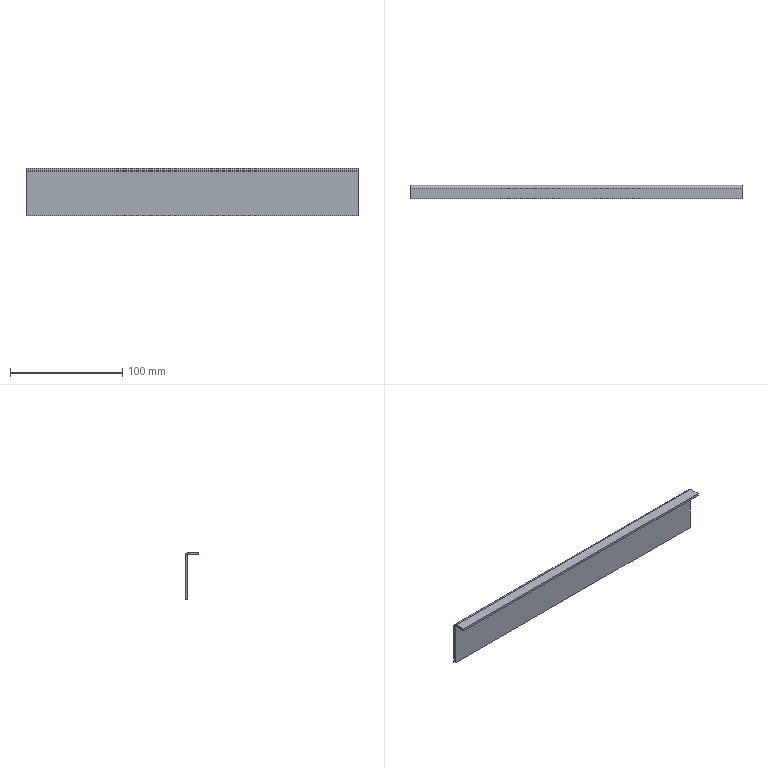Part | NX | 1 solid | 14 faces | box 296 x 12 x 42 mm | volume 30343 mm3 | plane 12 | cylinder 2 | commonest cylinder face diameters 1.473 x1 5.473 x1
STEP:
#1=CARTESIAN_POINT('',(-148.,-2.,-20.));
#2=VERTEX_POINT('',#1);
#3=CARTESIAN_POINT('',(-148.,-2.,19.263));
#4=VERTEX_POINT('',#3);
#5=CARTESIAN_POINT('',(-148.,-2.,20.));
#6=DIRECTION('',(0.,0.,1.));
#7=VECTOR('',#6,1000.);
#8=LINE('',#5,#7);
#9=EDGE_CURVE('',#2,#4,#8,.T.);
#10=ORIENTED_EDGE('',*,*,#9,.T.);
#11=CARTESIAN_POINT('',(-148.,0.,19.263));
#12=VERTEX_POINT('',#11);
#13=CARTESIAN_POINT('',(-148.,-2.,19.263));
#14=DIRECTION('',(0.,1.,0.));
#15=VECTOR('',#14,1000.);
#16=LINE('',#13,#15);
#17=EDGE_CURVE('',#4,#12,#16,.T.);
#18=ORIENTED_EDGE('',*,*,#17,.T.);
#19=CARTESIAN_POINT('',(-148.,0.,-20.));
#20=VERTEX_POINT('',#19);
#21=CARTESIAN_POINT('',(-148.,0.,20.));
#22=DIRECTION('',(0.,0.,1.));
#23=VECTOR('',#22,1000.);
#24=LINE('',#21,#23);
#25=EDGE_CURVE('',#20,#12,#24,.T.);
#26=ORIENTED_EDGE('',*,*,#25,.F.);
#27=CARTESIAN_POINT('',(-148.,-2.,-20.));
#28=DIRECTION('',(0.,1.,0.));
#29=VECTOR('',#28,1000.);
#30=LINE('',#27,#29);
#31=EDGE_CURVE('',#2,#20,#30,.T.);
#32=ORIENTED_EDGE('',*,*,#31,.F.);
#33=EDGE_LOOP('',(#10,#18,#26,#32));
#34=FACE_BOUND('',#33,.T.);
#35=CARTESIAN_POINT('',(-148.,-2.,20.));
#36=DIRECTION('',(-1.,0.,0.));
#37=DIRECTION('',(0.,0.,1.));
#38=AXIS2_PLACEMENT_3D('',#35,#36,#37);
#39=PLANE('',#38);
#40=ADVANCED_FACE('',(#34),#39,.T.);
#41=CARTESIAN_POINT('',(148.,-2.,19.263));
#42=VERTEX_POINT('',#41);
#43=CARTESIAN_POINT('',(148.,-2.,-20.));
#44=VERTEX_POINT('',#43);
#45=CARTESIAN_POINT('',(148.,-2.,20.));
#46=DIRECTION('',(0.,0.,-1.));
#47=VECTOR('',#46,1000.);
#48=LINE('',#45,#47);
#49=EDGE_CURVE('',#42,#44,#48,.T.);
#50=ORIENTED_EDGE('',*,*,#49,.F.);
#51=CARTESIAN_POINT('',(-148.,-2.,19.263));
#52=DIRECTION('',(-1.,0.,0.));
#53=VECTOR('',#52,1000.);
#54=LINE('',#51,#53);
#55=EDGE_CURVE('',#4,#42,#54,.F.);
#56=ORIENTED_EDGE('',*,*,#55,.F.);
#57=ORIENTED_EDGE('',*,*,#9,.F.);
#58=CARTESIAN_POINT('',(-148.,-2.,-20.));
#59=DIRECTION('',(-1.,0.,0.));
#60=VECTOR('',#59,1000.);
#61=LINE('',#58,#60);
#62=EDGE_CURVE('',#44,#2,#61,.T.);
#63=ORIENTED_EDGE('',*,*,#62,.F.);
#64=EDGE_LOOP('',(#50,#56,#57,#63));
#65=FACE_BOUND('',#64,.T.);
#66=CARTESIAN_POINT('',(0.,-2.,0.));
#67=DIRECTION('',(0.,-1.,0.));
#68=DIRECTION('',(0.,0.,-1.));
#69=AXIS2_PLACEMENT_3D('',#66,#67,#68);
#70=PLANE('',#69);
#71=ADVANCED_FACE('',(#65),#70,.T.);
#72=CARTESIAN_POINT('',(148.,0.,19.263));
#73=VERTEX_POINT('',#72);
#74=CARTESIAN_POINT('',(-148.,0.,19.263));
#75=DIRECTION('',(-1.,0.,0.));
#76=VECTOR('',#75,1000.);
#77=LINE('',#74,#76);
#78=EDGE_CURVE('',#12,#73,#77,.F.);
#79=ORIENTED_EDGE('',*,*,#78,.T.);
#80=CARTESIAN_POINT('',(148.,0.,-20.));
#81=VERTEX_POINT('',#80);
#82=CARTESIAN_POINT('',(148.,0.,20.));
#83=DIRECTION('',(0.,0.,-1.));
#84=VECTOR('',#83,1000.);
#85=LINE('',#82,#84);
#86=EDGE_CURVE('',#73,#81,#85,.T.);
#87=ORIENTED_EDGE('',*,*,#86,.T.);
#88=CARTESIAN_POINT('',(-148.,0.,-20.));
#89=DIRECTION('',(-1.,0.,0.));
#90=VECTOR('',#89,1000.);
#91=LINE('',#88,#90);
#92=EDGE_CURVE('',#81,#20,#91,.T.);
#93=ORIENTED_EDGE('',*,*,#92,.T.);
#94=ORIENTED_EDGE('',*,*,#25,.T.);
#95=EDGE_LOOP('',(#79,#87,#93,#94));
#96=FACE_BOUND('',#95,.T.);
#97=CARTESIAN_POINT('',(0.,0.,0.));
#98=DIRECTION('',(0.,-1.,0.));
#99=DIRECTION('',(0.,0.,-1.));
#100=AXIS2_PLACEMENT_3D('',#97,#98,#99);
#101=PLANE('',#100);
#102=ADVANCED_FACE('',(#96),#101,.F.);
#103=CARTESIAN_POINT('',(148.,-2.,19.263));
#104=DIRECTION('',(0.,1.,0.));
#105=VECTOR('',#104,1000.);
#106=LINE('',#103,#105);
#107=EDGE_CURVE('',#42,#73,#106,.T.);
#108=ORIENTED_EDGE('',*,*,#107,.F.);
#109=ORIENTED_EDGE('',*,*,#49,.T.);
#110=CARTESIAN_POINT('',(148.,-2.,-20.));
#111=DIRECTION('',(0.,1.,0.));
#112=VECTOR('',#111,1000.);
#113=LINE('',#110,#112);
#114=EDGE_CURVE('',#44,#81,#113,.T.);
#115=ORIENTED_EDGE('',*,*,#114,.T.);
#116=ORIENTED_EDGE('',*,*,#86,.F.);
#117=EDGE_LOOP('',(#108,#109,#115,#116));
#118=FACE_BOUND('',#117,.T.);
#119=CARTESIAN_POINT('',(148.,-2.,20.));
#120=DIRECTION('',(1.,0.,0.));
#121=DIRECTION('',(0.,0.,-1.));
#122=AXIS2_PLACEMENT_3D('',#119,#120,#121);
#123=PLANE('',#122);
#124=ADVANCED_FACE('',(#118),#123,.T.);
#125=ORIENTED_EDGE('',*,*,#92,.F.);
#126=ORIENTED_EDGE('',*,*,#114,.F.);
#127=ORIENTED_EDGE('',*,*,#62,.T.);
#128=ORIENTED_EDGE('',*,*,#31,.T.);
#129=EDGE_LOOP('',(#125,#126,#127,#128));
#130=FACE_BOUND('',#129,.T.);
#131=CARTESIAN_POINT('',(-148.,-2.,-20.));
#132=DIRECTION('',(0.,0.,-1.));
#133=DIRECTION('',(-1.,0.,0.));
#134=AXIS2_PLACEMENT_3D('',#131,#132,#133);
#135=PLANE('',#134);
#136=ADVANCED_FACE('',(#130),#135,.T.);
#137=CARTESIAN_POINT('',(148.,-2.737,20.));
#138=VERTEX_POINT('',#137);
#139=CARTESIAN_POINT('',(148.,-2.737,22.));
#140=VERTEX_POINT('',#139);
#141=CARTESIAN_POINT('',(148.,-2.737,20.));
#142=DIRECTION('',(0.,0.,1.));
#143=VECTOR('',#142,1000.);
#144=LINE('',#141,#143);
#145=EDGE_CURVE('',#138,#140,#144,.T.);
#146=ORIENTED_EDGE('',*,*,#145,.F.);
#147=CARTESIAN_POINT('',(148.,-2.737,19.263));
#148=DIRECTION('',(-1.,0.,0.));
#149=DIRECTION('',(0.,0.,1.));
#150=AXIS2_PLACEMENT_3D('',#147,#148,#149);
#151=CIRCLE('',#150,0.7366);
#152=EDGE_CURVE('',#42,#138,#151,.F.);
#153=ORIENTED_EDGE('',*,*,#152,.F.);
#154=ORIENTED_EDGE('',*,*,#107,.T.);
#155=CARTESIAN_POINT('',(148.,-2.737,19.263));
#156=DIRECTION('',(-1.,0.,0.));
#157=DIRECTION('',(0.,0.,1.));
#158=AXIS2_PLACEMENT_3D('',#155,#156,#157);
#159=CIRCLE('',#158,2.737);
#160=EDGE_CURVE('',#73,#140,#159,.F.);
#161=ORIENTED_EDGE('',*,*,#160,.T.);
#162=EDGE_LOOP('',(#146,#153,#154,#161));
#163=FACE_BOUND('',#162,.T.);
#164=CARTESIAN_POINT('',(148.,-2.737,19.263));
#165=DIRECTION('',(1.,0.,0.));
#166=DIRECTION('',(0.,0.,-1.));
#167=AXIS2_PLACEMENT_3D('',#164,#165,#166);
#168=PLANE('',#167);
#169=ADVANCED_FACE('',(#163),#168,.T.);
#170=CARTESIAN_POINT('',(-148.,-2.737,20.));
#171=VERTEX_POINT('',#170);
#172=CARTESIAN_POINT('',(-148.,-2.737,19.263));
#173=DIRECTION('',(-1.,0.,0.));
#174=DIRECTION('',(0.,0.,1.));
#175=AXIS2_PLACEMENT_3D('',#172,#173,#174);
#176=CIRCLE('',#175,0.7366);
#177=EDGE_CURVE('',#171,#4,#176,.T.);
#178=ORIENTED_EDGE('',*,*,#177,.F.);
#179=CARTESIAN_POINT('',(-148.,-2.737,22.));
#180=VERTEX_POINT('',#179);
#181=CARTESIAN_POINT('',(-148.,-2.737,20.));
#182=DIRECTION('',(0.,0.,1.));
#183=VECTOR('',#182,1000.);
#184=LINE('',#181,#183);
#185=EDGE_CURVE('',#171,#180,#184,.T.);
#186=ORIENTED_EDGE('',*,*,#185,.T.);
#187=CARTESIAN_POINT('',(-148.,-2.737,19.263));
#188=DIRECTION('',(-1.,0.,0.));
#189=DIRECTION('',(0.,0.,1.));
#190=AXIS2_PLACEMENT_3D('',#187,#188,#189);
#191=CIRCLE('',#190,2.737);
#192=EDGE_CURVE('',#180,#12,#191,.T.);
#193=ORIENTED_EDGE('',*,*,#192,.T.);
#194=ORIENTED_EDGE('',*,*,#17,.F.);
#195=EDGE_LOOP('',(#178,#186,#193,#194));
#196=FACE_BOUND('',#195,.T.);
#197=CARTESIAN_POINT('',(-148.,-2.737,19.263));
#198=DIRECTION('',(1.,0.,0.));
#199=DIRECTION('',(0.,0.,-1.));
#200=AXIS2_PLACEMENT_3D('',#197,#198,#199);
#201=PLANE('',#200);
#202=ADVANCED_FACE('',(#196),#201,.F.);
#203=ORIENTED_EDGE('',*,*,#78,.F.);
#204=ORIENTED_EDGE('',*,*,#192,.F.);
#205=CARTESIAN_POINT('',(0.,-2.737,22.));
#206=DIRECTION('',(-1.,0.,0.));
#207=VECTOR('',#206,1000.);
#208=LINE('',#205,#207);
#209=EDGE_CURVE('',#140,#180,#208,.T.);
#210=ORIENTED_EDGE('',*,*,#209,.F.);
#211=ORIENTED_EDGE('',*,*,#160,.F.);
#212=EDGE_LOOP('',(#203,#204,#210,#211));
#213=FACE_BOUND('',#212,.T.);
#214=CARTESIAN_POINT('',(-148.,-2.737,19.263));
#215=DIRECTION('',(-1.,0.,0.));
#216=DIRECTION('',(0.,0.,1.));
#217=AXIS2_PLACEMENT_3D('',#214,#215,#216);
#218=CYLINDRICAL_SURFACE('',#217,2.737);
#219=ADVANCED_FACE('',(#213),#218,.T.);
#220=ORIENTED_EDGE('',*,*,#55,.T.);
#221=ORIENTED_EDGE('',*,*,#152,.T.);
#222=CARTESIAN_POINT('',(148.,-2.737,20.));
#223=DIRECTION('',(-1.,0.,0.));
#224=VECTOR('',#223,1000.);
#225=LINE('',#222,#224);
#226=EDGE_CURVE('',#138,#171,#225,.T.);
#227=ORIENTED_EDGE('',*,*,#226,.T.);
#228=ORIENTED_EDGE('',*,*,#177,.T.);
#229=EDGE_LOOP('',(#220,#221,#227,#228));
#230=FACE_BOUND('',#229,.T.);
#231=CARTESIAN_POINT('',(-148.,-2.737,19.263));
#232=DIRECTION('',(-1.,0.,0.));
#233=DIRECTION('',(0.,0.,1.));
#234=AXIS2_PLACEMENT_3D('',#231,#232,#233);
#235=CYLINDRICAL_SURFACE('',#234,0.7366);
#236=ADVANCED_FACE('',(#230),#235,.F.);
#237=CARTESIAN_POINT('',(-148.,-12.,22.));
#238=VERTEX_POINT('',#237);
#239=CARTESIAN_POINT('',(-148.,-2.,22.));
#240=DIRECTION('',(0.,1.,0.));
#241=VECTOR('',#240,1000.);
#242=LINE('',#239,#241);
#243=EDGE_CURVE('',#238,#180,#242,.T.);
#244=ORIENTED_EDGE('',*,*,#243,.T.);
#245=ORIENTED_EDGE('',*,*,#185,.F.);
#246=CARTESIAN_POINT('',(-148.,-12.,20.));
#247=VERTEX_POINT('',#246);
#248=CARTESIAN_POINT('',(-148.,-2.,20.));
#249=DIRECTION('',(0.,1.,0.));
#250=VECTOR('',#249,1000.);
#251=LINE('',#248,#250);
#252=EDGE_CURVE('',#247,#171,#251,.T.);
#253=ORIENTED_EDGE('',*,*,#252,.F.);
#254=CARTESIAN_POINT('',(-148.,-12.,22.));
#255=DIRECTION('',(0.,0.,-1.));
#256=VECTOR('',#255,1000.);
#257=LINE('',#254,#256);
#258=EDGE_CURVE('',#238,#247,#257,.T.);
#259=ORIENTED_EDGE('',*,*,#258,.F.);
#260=EDGE_LOOP('',(#244,#245,#253,#259));
#261=FACE_BOUND('',#260,.T.);
#262=CARTESIAN_POINT('',(-148.,-2.,22.));
#263=DIRECTION('',(-1.,0.,0.));
#264=DIRECTION('',(0.,0.,1.));
#265=AXIS2_PLACEMENT_3D('',#262,#263,#264);
#266=PLANE('',#265);
#267=ADVANCED_FACE('',(#261),#266,.T.);
#268=CARTESIAN_POINT('',(148.,-12.,20.));
#269=VERTEX_POINT('',#268);
#270=CARTESIAN_POINT('',(148.,-12.,20.));
#271=DIRECTION('',(0.,-1.,0.));
#272=VECTOR('',#271,1000.);
#273=LINE('',#270,#272);
#274=EDGE_CURVE('',#138,#269,#273,.T.);
#275=ORIENTED_EDGE('',*,*,#274,.F.);
#276=ORIENTED_EDGE('',*,*,#145,.T.);
#277=CARTESIAN_POINT('',(148.,-12.,22.));
#278=VERTEX_POINT('',#277);
#279=CARTESIAN_POINT('',(148.,-12.,22.));
#280=DIRECTION('',(0.,-1.,0.));
#281=VECTOR('',#280,1000.);
#282=LINE('',#279,#281);
#283=EDGE_CURVE('',#140,#278,#282,.T.);
#284=ORIENTED_EDGE('',*,*,#283,.T.);
#285=CARTESIAN_POINT('',(148.,-12.,22.));
#286=DIRECTION('',(0.,0.,-1.));
#287=VECTOR('',#286,1000.);
#288=LINE('',#285,#287);
#289=EDGE_CURVE('',#278,#269,#288,.T.);
#290=ORIENTED_EDGE('',*,*,#289,.T.);
#291=EDGE_LOOP('',(#275,#276,#284,#290));
#292=FACE_BOUND('',#291,.T.);
#293=CARTESIAN_POINT('',(148.,-12.,22.));
#294=DIRECTION('',(1.,0.,0.));
#295=DIRECTION('',(0.,0.,-1.));
#296=AXIS2_PLACEMENT_3D('',#293,#294,#295);
#297=PLANE('',#296);
#298=ADVANCED_FACE('',(#292),#297,.T.);
#299=ORIENTED_EDGE('',*,*,#283,.F.);
#300=ORIENTED_EDGE('',*,*,#209,.T.);
#301=ORIENTED_EDGE('',*,*,#243,.F.);
#302=CARTESIAN_POINT('',(-148.,-12.,22.));
#303=DIRECTION('',(-1.,0.,0.));
#304=VECTOR('',#303,1000.);
#305=LINE('',#302,#304);
#306=EDGE_CURVE('',#278,#238,#305,.T.);
#307=ORIENTED_EDGE('',*,*,#306,.F.);
#308=EDGE_LOOP('',(#299,#300,#301,#307));
#309=FACE_BOUND('',#308,.T.);
#310=CARTESIAN_POINT('',(0.,0.,22.));
#311=DIRECTION('',(0.,0.,1.));
#312=DIRECTION('',(0.,-1.,0.));
#313=AXIS2_PLACEMENT_3D('',#310,#311,#312);
#314=PLANE('',#313);
#315=ADVANCED_FACE('',(#309),#314,.T.);
#316=ORIENTED_EDGE('',*,*,#226,.F.);
#317=ORIENTED_EDGE('',*,*,#274,.T.);
#318=CARTESIAN_POINT('',(-148.,-12.,20.));
#319=DIRECTION('',(-1.,0.,0.));
#320=VECTOR('',#319,1000.);
#321=LINE('',#318,#320);
#322=EDGE_CURVE('',#269,#247,#321,.T.);
#323=ORIENTED_EDGE('',*,*,#322,.T.);
#324=ORIENTED_EDGE('',*,*,#252,.T.);
#325=EDGE_LOOP('',(#316,#317,#323,#324));
#326=FACE_BOUND('',#325,.T.);
#327=CARTESIAN_POINT('',(0.,0.,20.));
#328=DIRECTION('',(0.,0.,1.));
#329=DIRECTION('',(0.,-1.,0.));
#330=AXIS2_PLACEMENT_3D('',#327,#328,#329);
#331=PLANE('',#330);
#332=ADVANCED_FACE('',(#326),#331,.F.);
#333=ORIENTED_EDGE('',*,*,#322,.F.);
#334=ORIENTED_EDGE('',*,*,#289,.F.);
#335=ORIENTED_EDGE('',*,*,#306,.T.);
#336=ORIENTED_EDGE('',*,*,#258,.T.);
#337=EDGE_LOOP('',(#333,#334,#335,#336));
#338=FACE_BOUND('',#337,.T.);
#339=CARTESIAN_POINT('',(-148.,-12.,22.));
#340=DIRECTION('',(0.,-1.,0.));
#341=DIRECTION('',(0.,0.,-1.));
#342=AXIS2_PLACEMENT_3D('',#339,#340,#341);
#343=PLANE('',#342);
#344=ADVANCED_FACE('',(#338),#343,.T.);
#345=CLOSED_SHELL('',(#40,#71,#102,#124,#136,#169,#202,#219,#236,#267,#298,#315,#332,#344));
#346=MANIFOLD_SOLID_BREP('',#345);
#347=(LENGTH_UNIT()NAMED_UNIT(*)SI_UNIT(.MILLI.,.METRE.));
#348=UNCERTAINTY_MEASURE_WITH_UNIT(LENGTH_MEASURE(0.00001),#347,'','');
#349=(NAMED_UNIT(*)PLANE_ANGLE_UNIT()SI_UNIT($,.RADIAN.));
#350=(NAMED_UNIT(*)SI_UNIT($,.STERADIAN.)SOLID_ANGLE_UNIT());
#351=(GEOMETRIC_REPRESENTATION_CONTEXT(3)GLOBAL_UNCERTAINTY_ASSIGNED_CONTEXT((#348))GLOBAL_UNIT_ASSIGNED_CONTEXT((#347,#349,#350))REPRESENTATION_CONTEXT('',''));
#352=ADVANCED_BREP_SHAPE_REPRESENTATION('',(#346),#351);